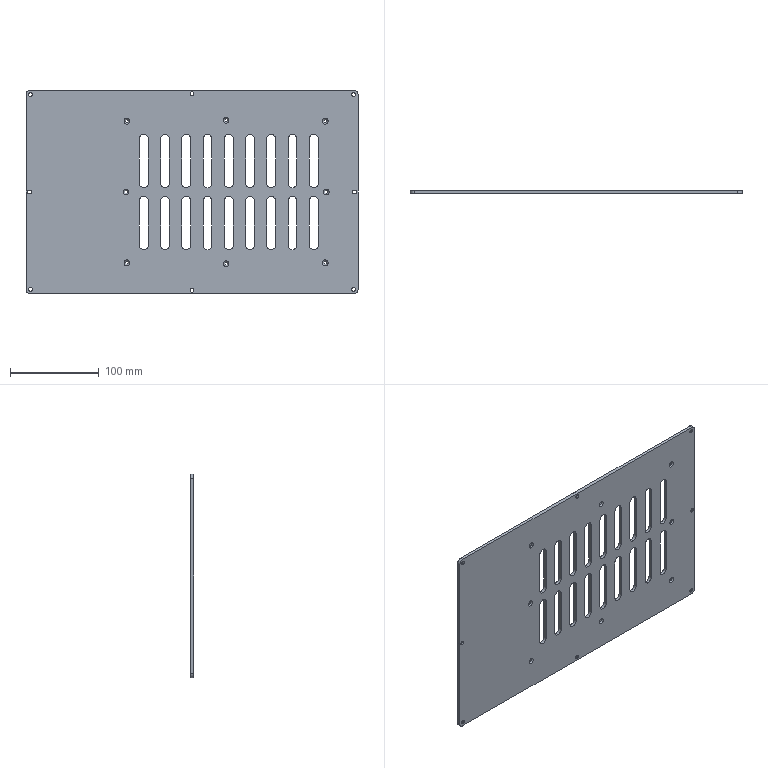Part | SolidWorks | features HoleWzd 2, MoveFace 2, BaseBody 1, Cut 1 | 1 solid | 164 faces | box 375 x 3.5 x 230 mm | volume 264309 mm3 | cylinder 90 | plane 42 | cone 32 | commonest cylinder face diameters 10 x58 3.5 x16 4.5 x16